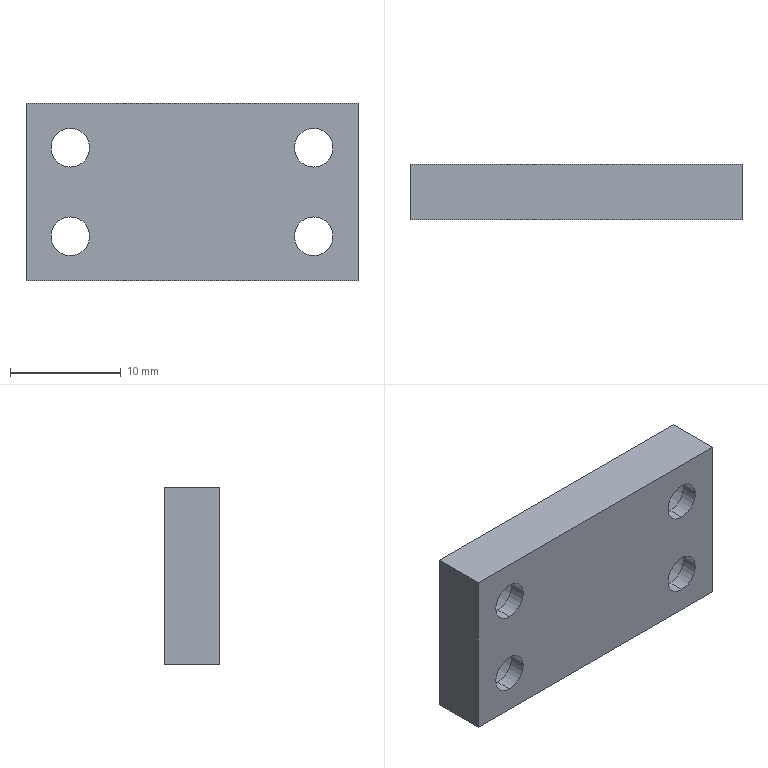Part | STEP file | 0246_207_Plate | 1 solid | 26 faces | box 30 x 5 x 16 mm | volume 1878 mm3 | cylinder 16 | plane 10 | commonest cylinder face diameters 3.5 x8 6.5 x8